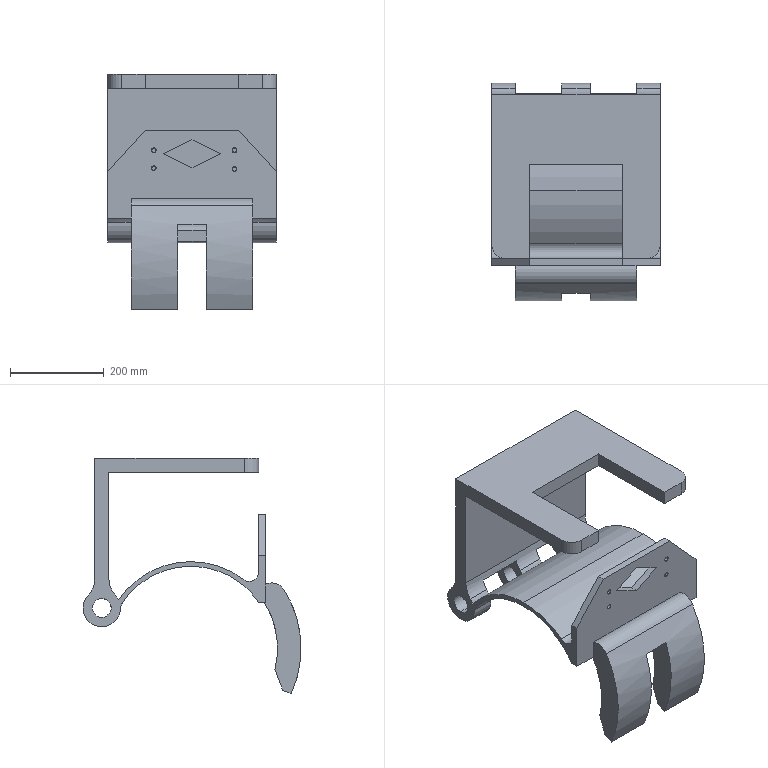Part | SolidWorks | features Cut 8, ICE 6, Fillet 5, BossThin 2, Chamfer 1, Extrusion 1, HoleWzd 1 | 1 solid | 85 faces | box 360 x 465.197 x 503.516 mm | volume 10385107 mm3 | cylinder 41 | plane 36 | cone 8 | commonest cylinder face diameters 8.5 x8 40 x8 80 x7 100 x5 10 x4 60 x3